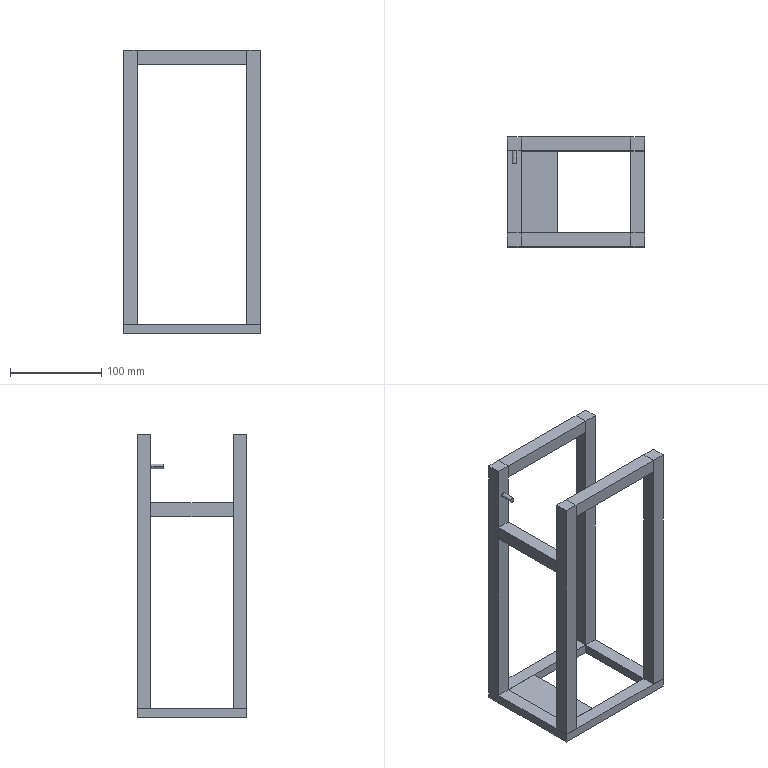Part | SolidWorks | features ICE 6, Extrusion 1 | 9 solids | 61 faces | box 150 x 120 x 310 mm | volume 427325 mm3 | plane 59 | cylinder 2 | commonest cylinder face diameters 5 x2
STEP:
#1=CARTESIAN_POINT('',(75.,-60.,0.));
#2=VERTEX_POINT('',#1);
#3=CARTESIAN_POINT('',(75.,60.,0.));
#4=VERTEX_POINT('',#3);
#5=CARTESIAN_POINT('',(75.,60.,0.));
#6=DIRECTION('',(0.,1.,0.));
#7=VECTOR('',#6,1000.);
#8=LINE('',#5,#7);
#9=EDGE_CURVE('',#2,#4,#8,.T.);
#10=ORIENTED_EDGE('',*,*,#9,.T.);
#11=CARTESIAN_POINT('',(75.,60.,10.));
#12=VERTEX_POINT('',#11);
#13=CARTESIAN_POINT('',(75.,60.,10.));
#14=DIRECTION('',(0.,0.,-1.));
#15=VECTOR('',#14,1000.);
#16=LINE('',#13,#15);
#17=EDGE_CURVE('',#12,#4,#16,.T.);
#18=ORIENTED_EDGE('',*,*,#17,.F.);
#19=CARTESIAN_POINT('',(75.,-60.,10.));
#20=VERTEX_POINT('',#19);
#21=CARTESIAN_POINT('',(75.,60.,10.));
#22=DIRECTION('',(0.,1.,0.));
#23=VECTOR('',#22,1000.);
#24=LINE('',#21,#23);
#25=EDGE_CURVE('',#20,#12,#24,.T.);
#26=ORIENTED_EDGE('',*,*,#25,.F.);
#27=CARTESIAN_POINT('',(75.,-60.,10.));
#28=DIRECTION('',(0.,0.,-1.));
#29=VECTOR('',#28,1000.);
#30=LINE('',#27,#29);
#31=EDGE_CURVE('',#20,#2,#30,.T.);
#32=ORIENTED_EDGE('',*,*,#31,.T.);
#33=EDGE_LOOP('',(#10,#18,#26,#32));
#34=FACE_OUTER_BOUND('',#33,.T.);
#35=CARTESIAN_POINT('',(75.,60.,10.));
#36=DIRECTION('',(-1.,0.,0.));
#37=DIRECTION('',(0.,-1.,0.));
#38=AXIS2_PLACEMENT_3D('',#35,#36,#37);
#39=PLANE('',#38);
#40=ADVANCED_FACE('',(#34),#39,.F.);
#41=CARTESIAN_POINT('',(-75.,60.,0.));
#42=VERTEX_POINT('',#41);
#43=CARTESIAN_POINT('',(-75.,60.,0.));
#44=DIRECTION('',(-1.,0.,0.));
#45=VECTOR('',#44,1000.);
#46=LINE('',#43,#45);
#47=EDGE_CURVE('',#4,#42,#46,.T.);
#48=ORIENTED_EDGE('',*,*,#47,.T.);
#49=CARTESIAN_POINT('',(-75.,60.,10.));
#50=VERTEX_POINT('',#49);
#51=CARTESIAN_POINT('',(-75.,60.,10.));
#52=DIRECTION('',(0.,0.,-1.));
#53=VECTOR('',#52,1000.);
#54=LINE('',#51,#53);
#55=EDGE_CURVE('',#50,#42,#54,.T.);
#56=ORIENTED_EDGE('',*,*,#55,.F.);
#57=CARTESIAN_POINT('',(-75.,60.,10.));
#58=DIRECTION('',(-1.,0.,0.));
#59=VECTOR('',#58,1000.);
#60=LINE('',#57,#59);
#61=EDGE_CURVE('',#12,#50,#60,.T.);
#62=ORIENTED_EDGE('',*,*,#61,.F.);
#63=ORIENTED_EDGE('',*,*,#17,.T.);
#64=EDGE_LOOP('',(#48,#56,#62,#63));
#65=FACE_OUTER_BOUND('',#64,.T.);
#66=CARTESIAN_POINT('',(-75.,60.,10.));
#67=DIRECTION('',(0.,-1.,0.));
#68=DIRECTION('',(0.,0.,-1.));
#69=AXIS2_PLACEMENT_3D('',#66,#67,#68);
#70=PLANE('',#69);
#71=ADVANCED_FACE('',(#65),#70,.F.);
#72=CARTESIAN_POINT('',(-75.,-60.,0.));
#73=VERTEX_POINT('',#72);
#74=CARTESIAN_POINT('',(-75.,60.,0.));
#75=DIRECTION('',(0.,-1.,0.));
#76=VECTOR('',#75,1000.);
#77=LINE('',#74,#76);
#78=EDGE_CURVE('',#42,#73,#77,.T.);
#79=ORIENTED_EDGE('',*,*,#78,.T.);
#80=CARTESIAN_POINT('',(-75.,-60.,10.));
#81=VERTEX_POINT('',#80);
#82=CARTESIAN_POINT('',(-75.,-60.,10.));
#83=DIRECTION('',(0.,0.,-1.));
#84=VECTOR('',#83,1000.);
#85=LINE('',#82,#84);
#86=EDGE_CURVE('',#81,#73,#85,.T.);
#87=ORIENTED_EDGE('',*,*,#86,.F.);
#88=CARTESIAN_POINT('',(-75.,60.,10.));
#89=DIRECTION('',(0.,-1.,0.));
#90=VECTOR('',#89,1000.);
#91=LINE('',#88,#90);
#92=EDGE_CURVE('',#50,#81,#91,.T.);
#93=ORIENTED_EDGE('',*,*,#92,.F.);
#94=ORIENTED_EDGE('',*,*,#55,.T.);
#95=EDGE_LOOP('',(#79,#87,#93,#94));
#96=FACE_OUTER_BOUND('',#95,.T.);
#97=CARTESIAN_POINT('',(-75.,60.,10.));
#98=DIRECTION('',(1.,0.,0.));
#99=DIRECTION('',(0.,1.,0.));
#100=AXIS2_PLACEMENT_3D('',#97,#98,#99);
#101=PLANE('',#100);
#102=ADVANCED_FACE('',(#96),#101,.F.);
#103=CARTESIAN_POINT('',(-75.,-60.,0.));
#104=DIRECTION('',(1.,0.,0.));
#105=VECTOR('',#104,1000.);
#106=LINE('',#103,#105);
#107=EDGE_CURVE('',#73,#2,#106,.T.);
#108=ORIENTED_EDGE('',*,*,#107,.T.);
#109=ORIENTED_EDGE('',*,*,#31,.F.);
#110=CARTESIAN_POINT('',(-75.,-60.,10.));
#111=DIRECTION('',(1.,0.,0.));
#112=VECTOR('',#111,1000.);
#113=LINE('',#110,#112);
#114=EDGE_CURVE('',#81,#20,#113,.T.);
#115=ORIENTED_EDGE('',*,*,#114,.F.);
#116=ORIENTED_EDGE('',*,*,#86,.T.);
#117=EDGE_LOOP('',(#108,#109,#115,#116));
#118=FACE_OUTER_BOUND('',#117,.T.);
#119=CARTESIAN_POINT('',(-75.,-60.,10.));
#120=DIRECTION('',(0.,1.,0.));
#121=DIRECTION('',(0.,0.,1.));
#122=AXIS2_PLACEMENT_3D('',#119,#120,#121);
#123=PLANE('',#122);
#124=ADVANCED_FACE('',(#118),#123,.F.);
#125=CARTESIAN_POINT('',(60.,-45.,10.));
#126=VERTEX_POINT('',#125);
#127=CARTESIAN_POINT('',(60.,45.,10.));
#128=VERTEX_POINT('',#127);
#129=CARTESIAN_POINT('',(60.,0.,10.));
#130=DIRECTION('',(0.,1.,0.));
#131=VECTOR('',#130,1000.);
#132=LINE('',#129,#131);
#133=EDGE_CURVE('',#126,#128,#132,.T.);
#134=ORIENTED_EDGE('',*,*,#133,.F.);
#135=CARTESIAN_POINT('',(-60.,-45.,10.));
#136=VERTEX_POINT('',#135);
#137=CARTESIAN_POINT('',(0.,-45.,10.));
#138=DIRECTION('',(1.,0.,0.));
#139=VECTOR('',#138,1000.);
#140=LINE('',#137,#139);
#141=EDGE_CURVE('',#136,#126,#140,.T.);
#142=ORIENTED_EDGE('',*,*,#141,.F.);
#143=CARTESIAN_POINT('',(-60.,45.,10.));
#144=VERTEX_POINT('',#143);
#145=CARTESIAN_POINT('',(-60.,0.,10.));
#146=DIRECTION('',(0.,-1.,0.));
#147=VECTOR('',#146,1000.);
#148=LINE('',#145,#147);
#149=EDGE_CURVE('',#144,#136,#148,.T.);
#150=ORIENTED_EDGE('',*,*,#149,.F.);
#151=CARTESIAN_POINT('',(0.,45.,10.));
#152=DIRECTION('',(-1.,0.,0.));
#153=VECTOR('',#152,1000.);
#154=LINE('',#151,#153);
#155=EDGE_CURVE('',#128,#144,#154,.T.);
#156=ORIENTED_EDGE('',*,*,#155,.F.);
#157=EDGE_LOOP('',(#134,#142,#150,#156));
#158=FACE_BOUND('',#157,.T.);
#159=ORIENTED_EDGE('',*,*,#25,.T.);
#160=ORIENTED_EDGE('',*,*,#61,.T.);
#161=ORIENTED_EDGE('',*,*,#92,.T.);
#162=ORIENTED_EDGE('',*,*,#114,.T.);
#163=EDGE_LOOP('',(#159,#160,#161,#162));
#164=FACE_OUTER_BOUND('',#163,.T.);
#165=CARTESIAN_POINT('',(0.,0.,10.));
#166=DIRECTION('',(0.,0.,1.));
#167=DIRECTION('',(1.,0.,0.));
#168=AXIS2_PLACEMENT_3D('',#165,#166,#167);
#169=PLANE('',#168);
#170=ADVANCED_FACE('',(#158,#164),#169,.T.);
#171=CARTESIAN_POINT('',(-60.,-45.,0.));
#172=VERTEX_POINT('',#171);
#173=CARTESIAN_POINT('',(60.,-45.,0.));
#174=VERTEX_POINT('',#173);
#175=CARTESIAN_POINT('',(-60.,-45.,0.));
#176=DIRECTION('',(1.,0.,0.));
#177=VECTOR('',#176,1000.);
#178=LINE('',#175,#177);
#179=EDGE_CURVE('',#172,#174,#178,.T.);
#180=ORIENTED_EDGE('',*,*,#179,.T.);
#181=CARTESIAN_POINT('',(60.,45.,0.));
#182=VERTEX_POINT('',#181);
#183=CARTESIAN_POINT('',(60.,45.,0.));
#184=DIRECTION('',(0.,1.,0.));
#185=VECTOR('',#184,1000.);
#186=LINE('',#183,#185);
#187=EDGE_CURVE('',#174,#182,#186,.T.);
#188=ORIENTED_EDGE('',*,*,#187,.T.);
#189=CARTESIAN_POINT('',(-60.,45.,0.));
#190=VERTEX_POINT('',#189);
#191=CARTESIAN_POINT('',(-60.,45.,0.));
#192=DIRECTION('',(-1.,0.,0.));
#193=VECTOR('',#192,1000.);
#194=LINE('',#191,#193);
#195=EDGE_CURVE('',#182,#190,#194,.T.);
#196=ORIENTED_EDGE('',*,*,#195,.T.);
#197=CARTESIAN_POINT('',(-60.,45.,0.));
#198=DIRECTION('',(0.,-1.,0.));
#199=VECTOR('',#198,1000.);
#200=LINE('',#197,#199);
#201=EDGE_CURVE('',#190,#172,#200,.T.);
#202=ORIENTED_EDGE('',*,*,#201,.T.);
#203=EDGE_LOOP('',(#180,#188,#196,#202));
#204=FACE_BOUND('',#203,.T.);
#205=ORIENTED_EDGE('',*,*,#9,.F.);
#206=ORIENTED_EDGE('',*,*,#107,.F.);
#207=ORIENTED_EDGE('',*,*,#78,.F.);
#208=ORIENTED_EDGE('',*,*,#47,.F.);
#209=EDGE_LOOP('',(#205,#206,#207,#208));
#210=FACE_OUTER_BOUND('',#209,.T.);
#211=CARTESIAN_POINT('',(0.,0.,0.));
#212=DIRECTION('',(0.,0.,1.));
#213=DIRECTION('',(1.,0.,0.));
#214=AXIS2_PLACEMENT_3D('',#211,#212,#213);
#215=PLANE('',#214);
#216=ADVANCED_FACE('',(#204,#210),#215,.F.);
#217=ORIENTED_EDGE('',*,*,#133,.T.);
#218=CARTESIAN_POINT('',(60.,45.,0.));
#219=DIRECTION('',(0.,0.,1.));
#220=VECTOR('',#219,1000.);
#221=LINE('',#218,#220);
#222=EDGE_CURVE('',#182,#128,#221,.T.);
#223=ORIENTED_EDGE('',*,*,#222,.F.);
#224=ORIENTED_EDGE('',*,*,#187,.F.);
#225=CARTESIAN_POINT('',(60.,-45.,0.));
#226=DIRECTION('',(0.,0.,1.));
#227=VECTOR('',#226,1000.);
#228=LINE('',#225,#227);
#229=EDGE_CURVE('',#174,#126,#228,.T.);
#230=ORIENTED_EDGE('',*,*,#229,.T.);
#231=EDGE_LOOP('',(#217,#223,#224,#230));
#232=FACE_OUTER_BOUND('',#231,.T.);
#233=CARTESIAN_POINT('',(60.,45.,0.));
#234=DIRECTION('',(1.,0.,0.));
#235=DIRECTION('',(0.,0.,-1.));
#236=AXIS2_PLACEMENT_3D('',#233,#234,#235);
#237=PLANE('',#236);
#238=ADVANCED_FACE('',(#232),#237,.F.);
#239=ORIENTED_EDGE('',*,*,#141,.T.);
#240=ORIENTED_EDGE('',*,*,#229,.F.);
#241=ORIENTED_EDGE('',*,*,#179,.F.);
#242=CARTESIAN_POINT('',(-60.,-45.,0.));
#243=DIRECTION('',(0.,0.,1.));
#244=VECTOR('',#243,1000.);
#245=LINE('',#242,#244);
#246=EDGE_CURVE('',#172,#136,#245,.T.);
#247=ORIENTED_EDGE('',*,*,#246,.T.);
#248=EDGE_LOOP('',(#239,#240,#241,#247));
#249=FACE_OUTER_BOUND('',#248,.T.);
#250=CARTESIAN_POINT('',(-60.,-45.,0.));
#251=DIRECTION('',(0.,-1.,0.));
#252=DIRECTION('',(0.,0.,-1.));
#253=AXIS2_PLACEMENT_3D('',#250,#251,#252);
#254=PLANE('',#253);
#255=ADVANCED_FACE('',(#249),#254,.F.);
#256=ORIENTED_EDGE('',*,*,#149,.T.);
#257=ORIENTED_EDGE('',*,*,#246,.F.);
#258=ORIENTED_EDGE('',*,*,#201,.F.);
#259=CARTESIAN_POINT('',(-60.,45.,0.));
#260=DIRECTION('',(0.,0.,1.));
#261=VECTOR('',#260,1000.);
#262=LINE('',#259,#261);
#263=EDGE_CURVE('',#190,#144,#262,.T.);
#264=ORIENTED_EDGE('',*,*,#263,.T.);
#265=EDGE_LOOP('',(#256,#257,#258,#264));
#266=FACE_OUTER_BOUND('',#265,.T.);
#267=CARTESIAN_POINT('',(-60.,45.,0.));
#268=DIRECTION('',(-1.,0.,0.));
#269=DIRECTION('',(0.,0.,1.));
#270=AXIS2_PLACEMENT_3D('',#267,#268,#269);
#271=PLANE('',#270);
#272=ADVANCED_FACE('',(#266),#271,.F.);
#273=ORIENTED_EDGE('',*,*,#155,.T.);
#274=ORIENTED_EDGE('',*,*,#263,.F.);
#275=ORIENTED_EDGE('',*,*,#195,.F.);
#276=ORIENTED_EDGE('',*,*,#222,.T.);
#277=EDGE_LOOP('',(#273,#274,#275,#276));
#278=FACE_OUTER_BOUND('',#277,.T.);
#279=CARTESIAN_POINT('',(-60.,45.,0.));
#280=DIRECTION('',(0.,1.,0.));
#281=DIRECTION('',(0.,0.,1.));
#282=AXIS2_PLACEMENT_3D('',#279,#280,#281);
#283=PLANE('',#282);
#284=ADVANCED_FACE('',(#278),#283,.F.);
#285=CLOSED_SHELL('',(#40,#71,#102,#124,#170,#216,#238,#255,#272,#284));
#286=MANIFOLD_SOLID_BREP('',#285);
#287=CARTESIAN_POINT('',(-75.,-45.,10.));
#288=VERTEX_POINT('',#287);
#289=CARTESIAN_POINT('',(-75.,-60.,10.));
#290=VERTEX_POINT('',#289);
#291=CARTESIAN_POINT('',(-75.,-60.,10.));
#292=DIRECTION('',(0.,-1.,0.));
#293=VECTOR('',#292,1000.);
#294=LINE('',#291,#293);
#295=EDGE_CURVE('',#288,#290,#294,.T.);
#296=ORIENTED_EDGE('',*,*,#295,.T.);
#297=CARTESIAN_POINT('',(-75.,-60.,310.));
#298=VERTEX_POINT('',#297);
#299=CARTESIAN_POINT('',(-75.,-60.,310.));
#300=DIRECTION('',(0.,0.,-1.));
#301=VECTOR('',#300,1000.);
#302=LINE('',#299,#301);
#303=EDGE_CURVE('',#298,#290,#302,.T.);
#304=ORIENTED_EDGE('',*,*,#303,.F.);
#305=CARTESIAN_POINT('',(-75.,-45.,310.));
#306=VERTEX_POINT('',#305);
#307=CARTESIAN_POINT('',(-75.,-60.,310.));
#308=DIRECTION('',(0.,-1.,0.));
#309=VECTOR('',#308,1000.);
#310=LINE('',#307,#309);
#311=EDGE_CURVE('',#306,#298,#310,.T.);
#312=ORIENTED_EDGE('',*,*,#311,.F.);
#313=CARTESIAN_POINT('',(-75.,-45.,310.));
#314=DIRECTION('',(0.,0.,-1.));
#315=VECTOR('',#314,1000.);
#316=LINE('',#313,#315);
#317=EDGE_CURVE('',#306,#288,#316,.T.);
#318=ORIENTED_EDGE('',*,*,#317,.T.);
#319=EDGE_LOOP('',(#296,#304,#312,#318));
#320=FACE_OUTER_BOUND('',#319,.T.);
#321=CARTESIAN_POINT('',(-75.,-60.,310.));
#322=DIRECTION('',(1.,0.,0.));
#323=DIRECTION('',(0.,0.,-1.));
#324=AXIS2_PLACEMENT_3D('',#321,#322,#323);
#325=PLANE('',#324);
#326=ADVANCED_FACE('',(#320),#325,.F.);
#327=CARTESIAN_POINT('',(-60.,-60.,10.));
#328=VERTEX_POINT('',#327);
#329=CARTESIAN_POINT('',(-75.,-60.,10.));
#330=DIRECTION('',(1.,0.,0.));
#331=VECTOR('',#330,1000.);
#332=LINE('',#329,#331);
#333=EDGE_CURVE('',#290,#328,#332,.T.);
#334=ORIENTED_EDGE('',*,*,#333,.T.);
#335=CARTESIAN_POINT('',(-60.,-60.,310.));
#336=VERTEX_POINT('',#335);
#337=CARTESIAN_POINT('',(-60.,-60.,310.));
#338=DIRECTION('',(0.,0.,-1.));
#339=VECTOR('',#338,1000.);
#340=LINE('',#337,#339);
#341=EDGE_CURVE('',#336,#328,#340,.T.);
#342=ORIENTED_EDGE('',*,*,#341,.F.);
#343=CARTESIAN_POINT('',(-75.,-60.,310.));
#344=DIRECTION('',(1.,0.,0.));
#345=VECTOR('',#344,1000.);
#346=LINE('',#343,#345);
#347=EDGE_CURVE('',#298,#336,#346,.T.);
#348=ORIENTED_EDGE('',*,*,#347,.F.);
#349=ORIENTED_EDGE('',*,*,#303,.T.);
#350=EDGE_LOOP('',(#334,#342,#348,#349));
#351=FACE_OUTER_BOUND('',#350,.T.);
#352=CARTESIAN_POINT('',(-75.,-60.,310.));
#353=DIRECTION('',(0.,1.,0.));
#354=DIRECTION('',(0.,0.,1.));
#355=AXIS2_PLACEMENT_3D('',#352,#353,#354);
#356=PLANE('',#355);
#357=ADVANCED_FACE('',(#351),#356,.F.);
#358=CARTESIAN_POINT('',(-60.,-45.,10.));
#359=VERTEX_POINT('',#358);
#360=CARTESIAN_POINT('',(-60.,-60.,10.));
#361=DIRECTION('',(0.,1.,0.));
#362=VECTOR('',#361,1000.);
#363=LINE('',#360,#362);
#364=EDGE_CURVE('',#328,#359,#363,.T.);
#365=ORIENTED_EDGE('',*,*,#364,.T.);
#366=CARTESIAN_POINT('',(-60.,-45.,310.));
#367=VERTEX_POINT('',#366);
#368=CARTESIAN_POINT('',(-60.,-45.,310.));
#369=DIRECTION('',(0.,0.,-1.));
#370=VECTOR('',#369,1000.);
#371=LINE('',#368,#370);
#372=EDGE_CURVE('',#367,#359,#371,.T.);
#373=ORIENTED_EDGE('',*,*,#372,.F.);
#374=CARTESIAN_POINT('',(-60.,-60.,310.));
#375=DIRECTION('',(0.,1.,0.));
#376=VECTOR('',#375,1000.);
#377=LINE('',#374,#376);
#378=EDGE_CURVE('',#336,#367,#377,.T.);
#379=ORIENTED_EDGE('',*,*,#378,.F.);
#380=ORIENTED_EDGE('',*,*,#341,.T.);
#381=EDGE_LOOP('',(#365,#373,#379,#380));
#382=FACE_OUTER_BOUND('',#381,.T.);
#383=CARTESIAN_POINT('',(-60.,-60.,310.));
#384=DIRECTION('',(-1.,0.,0.));
#385=DIRECTION('',(0.,0.,1.));
#386=AXIS2_PLACEMENT_3D('',#383,#384,#385);
#387=PLANE('',#386);
#388=ADVANCED_FACE('',(#382),#387,.F.);
#389=CARTESIAN_POINT('',(-75.,-45.,10.));
#390=DIRECTION('',(-1.,0.,0.));
#391=VECTOR('',#390,1000.);
#392=LINE('',#389,#391);
#393=EDGE_CURVE('',#359,#288,#392,.T.);
#394=ORIENTED_EDGE('',*,*,#393,.T.);
#395=ORIENTED_EDGE('',*,*,#317,.F.);
#396=CARTESIAN_POINT('',(-75.,-45.,310.));
#397=DIRECTION('',(-1.,0.,0.));
#398=VECTOR('',#397,1000.);
#399=LINE('',#396,#398);
#400=EDGE_CURVE('',#367,#306,#399,.T.);
#401=ORIENTED_EDGE('',*,*,#400,.F.);
#402=ORIENTED_EDGE('',*,*,#372,.T.);
#403=EDGE_LOOP('',(#394,#395,#401,#402));
#404=FACE_OUTER_BOUND('',#403,.T.);
#405=CARTESIAN_POINT('',(-75.,-45.,310.));
#406=DIRECTION('',(0.,-1.,0.));
#407=DIRECTION('',(1.,0.,0.));
#408=AXIS2_PLACEMENT_3D('',#405,#406,#407);
#409=PLANE('',#408);
#410=ADVANCED_FACE('',(#404),#409,.F.);
#411=ORIENTED_EDGE('',*,*,#311,.T.);
#412=ORIENTED_EDGE('',*,*,#347,.T.);
#413=ORIENTED_EDGE('',*,*,#378,.T.);
#414=ORIENTED_EDGE('',*,*,#400,.T.);
#415=EDGE_LOOP('',(#411,#412,#413,#414));
#416=FACE_OUTER_BOUND('',#415,.T.);
#417=CARTESIAN_POINT('',(0.,0.,310.));
#418=DIRECTION('',(0.,0.,-1.));
#419=DIRECTION('',(-1.,0.,0.));
#420=AXIS2_PLACEMENT_3D('',#417,#418,#419);
#421=PLANE('',#420);
#422=ADVANCED_FACE('',(#416),#421,.F.);
#423=ORIENTED_EDGE('',*,*,#295,.F.);
#424=ORIENTED_EDGE('',*,*,#393,.F.);
#425=ORIENTED_EDGE('',*,*,#364,.F.);
#426=ORIENTED_EDGE('',*,*,#333,.F.);
#427=EDGE_LOOP('',(#423,#424,#425,#426));
#428=FACE_OUTER_BOUND('',#427,.T.);
#429=CARTESIAN_POINT('',(0.,0.,10.));
#430=DIRECTION('',(0.,0.,-1.));
#431=DIRECTION('',(-1.,0.,0.));
#432=AXIS2_PLACEMENT_3D('',#429,#430,#431);
#433=PLANE('',#432);
#434=ADVANCED_FACE('',(#428),#433,.T.);
#435=CLOSED_SHELL('',(#326,#357,#388,#410,#422,#434));
#436=MANIFOLD_SOLID_BREP('',#435);
#437=CARTESIAN_POINT('',(75.,45.,10.));
#438=VERTEX_POINT('',#437);
#439=CARTESIAN_POINT('',(75.,60.,10.));
#440=VERTEX_POINT('',#439);
#441=CARTESIAN_POINT('',(75.,60.,10.));
#442=DIRECTION('',(0.,1.,0.));
#443=VECTOR('',#442,1000.);
#444=LINE('',#441,#443);
#445=EDGE_CURVE('',#438,#440,#444,.T.);
#446=ORIENTED_EDGE('',*,*,#445,.T.);
#447=CARTESIAN_POINT('',(75.,60.,310.));
#448=VERTEX_POINT('',#447);
#449=CARTESIAN_POINT('',(75.,60.,310.));
#450=DIRECTION('',(0.,0.,-1.));
#451=VECTOR('',#450,1000.);
#452=LINE('',#449,#451);
#453=EDGE_CURVE('',#448,#440,#452,.T.);
#454=ORIENTED_EDGE('',*,*,#453,.F.);
#455=CARTESIAN_POINT('',(75.,45.,310.));
#456=VERTEX_POINT('',#455);
#457=CARTESIAN_POINT('',(75.,60.,310.));
#458=DIRECTION('',(0.,1.,0.));
#459=VECTOR('',#458,1000.);
#460=LINE('',#457,#459);
#461=EDGE_CURVE('',#456,#448,#460,.T.);
#462=ORIENTED_EDGE('',*,*,#461,.F.);
#463=CARTESIAN_POINT('',(75.,45.,310.));
#464=DIRECTION('',(0.,0.,-1.));
#465=VECTOR('',#464,1000.);
#466=LINE('',#463,#465);
#467=EDGE_CURVE('',#456,#438,#466,.T.);
#468=ORIENTED_EDGE('',*,*,#467,.T.);
#469=EDGE_LOOP('',(#446,#454,#462,#468));
#470=FACE_OUTER_BOUND('',#469,.T.);
#471=CARTESIAN_POINT('',(75.,60.,310.));
#472=DIRECTION('',(-1.,0.,0.));
#473=DIRECTION('',(0.,-1.,0.));
#474=AXIS2_PLACEMENT_3D('',#471,#472,#473);
#475=PLANE('',#474);
#476=ADVANCED_FACE('',(#470),#475,.F.);
#477=CARTESIAN_POINT('',(60.,60.,10.));
#478=VERTEX_POINT('',#477);
#479=CARTESIAN_POINT('',(75.,60.,10.));
#480=DIRECTION('',(-1.,0.,0.));
#481=VECTOR('',#480,1000.);
#482=LINE('',#479,#481);
#483=EDGE_CURVE('',#440,#478,#482,.T.);
#484=ORIENTED_EDGE('',*,*,#483,.T.);
#485=CARTESIAN_POINT('',(60.,60.,310.));
#486=VERTEX_POINT('',#485);
#487=CARTESIAN_POINT('',(60.,60.,310.));
#488=DIRECTION('',(0.,0.,-1.));
#489=VECTOR('',#488,1000.);
#490=LINE('',#487,#489);
#491=EDGE_CURVE('',#486,#478,#490,.T.);
#492=ORIENTED_EDGE('',*,*,#491,.F.);
#493=CARTESIAN_POINT('',(75.,60.,310.));
#494=DIRECTION('',(-1.,0.,0.));
#495=VECTOR('',#494,1000.);
#496=LINE('',#493,#495);
#497=EDGE_CURVE('',#448,#486,#496,.T.);
#498=ORIENTED_EDGE('',*,*,#497,.F.);
#499=ORIENTED_EDGE('',*,*,#453,.T.);
#500=EDGE_LOOP('',(#484,#492,#498,#499));
#501=FACE_OUTER_BOUND('',#500,.T.);
#502=CARTESIAN_POINT('',(75.,60.,310.));
#503=DIRECTION('',(0.,-1.,0.));
#504=DIRECTION('',(0.,0.,-1.));
#505=AXIS2_PLACEMENT_3D('',#502,#503,#504);
#506=PLANE('',#505);
#507=ADVANCED_FACE('',(#501),#506,.F.);
#508=CARTESIAN_POINT('',(60.,45.,10.));
#509=VERTEX_POINT('',#508);
#510=CARTESIAN_POINT('',(60.,60.,10.));
#511=DIRECTION('',(0.,-1.,0.));
#512=VECTOR('',#511,1000.);
#513=LINE('',#510,#512);
#514=EDGE_CURVE('',#478,#509,#513,.T.);
#515=ORIENTED_EDGE('',*,*,#514,.T.);
#516=CARTESIAN_POINT('',(60.,45.,310.));
#517=VERTEX_POINT('',#516);
#518=CARTESIAN_POINT('',(60.,45.,310.));
#519=DIRECTION('',(0.,0.,-1.));
#520=VECTOR('',#519,1000.);
#521=LINE('',#518,#520);
#522=EDGE_CURVE('',#517,#509,#521,.T.);
#523=ORIENTED_EDGE('',*,*,#522,.F.);
#524=CARTESIAN_POINT('',(60.,60.,310.));
#525=DIRECTION('',(0.,-1.,0.));
#526=VECTOR('',#525,1000.);
#527=LINE('',#524,#526);
#528=EDGE_CURVE('',#486,#517,#527,.T.);
#529=ORIENTED_EDGE('',*,*,#528,.F.);
#530=ORIENTED_EDGE('',*,*,#491,.T.);
#531=EDGE_LOOP('',(#515,#523,#529,#530));
#532=FACE_OUTER_BOUND('',#531,.T.);
#533=CARTESIAN_POINT('',(60.,60.,310.));
#534=DIRECTION('',(1.,0.,0.));
#535=DIRECTION('',(0.,1.,0.));
#536=AXIS2_PLACEMENT_3D('',#533,#534,#535);
#537=PLANE('',#536);
#538=ADVANCED_FACE('',(#532),#537,.F.);
#539=CARTESIAN_POINT('',(75.,45.,10.));
#540=DIRECTION('',(1.,0.,0.));
#541=VECTOR('',#540,1000.);
#542=LINE('',#539,#541);
#543=EDGE_CURVE('',#509,#438,#542,.T.);
#544=ORIENTED_EDGE('',*,*,#543,.T.);
#545=ORIENTED_EDGE('',*,*,#467,.F.);
#546=CARTESIAN_POINT('',(75.,45.,310.));
#547=DIRECTION('',(1.,0.,0.));
#548=VECTOR('',#547,1000.);
#549=LINE('',#546,#548);
#550=EDGE_CURVE('',#517,#456,#549,.T.);
#551=ORIENTED_EDGE('',*,*,#550,.F.);
#552=ORIENTED_EDGE('',*,*,#522,.T.);
#553=EDGE_LOOP('',(#544,#545,#551,#552));
#554=FACE_OUTER_BOUND('',#553,.T.);
#555=CARTESIAN_POINT('',(75.,45.,310.));
#556=DIRECTION('',(0.,1.,0.));
#557=DIRECTION('',(0.,0.,1.));
#558=AXIS2_PLACEMENT_3D('',#555,#556,#557);
#559=PLANE('',#558);
#560=ADVANCED_FACE('',(#554),#559,.F.);
#561=ORIENTED_EDGE('',*,*,#461,.T.);
#562=ORIENTED_EDGE('',*,*,#497,.T.);
#563=ORIENTED_EDGE('',*,*,#528,.T.);
#564=ORIENTED_EDGE('',*,*,#550,.T.);
#565=EDGE_LOOP('',(#561,#562,#563,#564));
#566=FACE_OUTER_BOUND('',#565,.T.);
#567=CARTESIAN_POINT('',(0.,0.,310.));
#568=DIRECTION('',(0.,0.,-1.));
#569=DIRECTION('',(-1.,0.,0.));
#570=AXIS2_PLACEMENT_3D('',#567,#568,#569);
#571=PLANE('',#570);
#572=ADVANCED_FACE('',(#566),#571,.F.);
#573=ORIENTED_EDGE('',*,*,#445,.F.);
#574=ORIENTED_EDGE('',*,*,#543,.F.);
#575=ORIENTED_EDGE('',*,*,#514,.F.);
#576=ORIENTED_EDGE('',*,*,#483,.F.);
#577=EDGE_LOOP('',(#573,#574,#575,#576));
#578=FACE_OUTER_BOUND('',#577,.T.);
#579=CARTESIAN_POINT('',(0.,0.,10.));
#580=DIRECTION('',(0.,0.,-1.));
#581=DIRECTION('',(-1.,0.,0.));
#582=AXIS2_PLACEMENT_3D('',#579,#580,#581);
#583=PLANE('',#582);
#584=ADVANCED_FACE('',(#578),#583,.T.);
#585=CLOSED_SHELL('',(#476,#507,#538,#560,#572,#584));
#586=MANIFOLD_SOLID_BREP('',#585);
#587=CARTESIAN_POINT('',(75.,-60.,10.));
#588=VERTEX_POINT('',#587);
#589=CARTESIAN_POINT('',(75.,-45.,10.));
#590=VERTEX_POINT('',#589);
#591=CARTESIAN_POINT('',(75.,-60.,10.));
#592=DIRECTION('',(0.,1.,0.));
#593=VECTOR('',#592,1000.);
#594=LINE('',#591,#593);
#595=EDGE_CURVE('',#588,#590,#594,.T.);
#596=ORIENTED_EDGE('',*,*,#595,.T.);
#597=CARTESIAN_POINT('',(75.,-45.,310.));
#598=VERTEX_POINT('',#597);
#599=CARTESIAN_POINT('',(75.,-45.,310.));
#600=DIRECTION('',(0.,0.,-1.));
#601=VECTOR('',#600,1000.);
#602=LINE('',#599,#601);
#603=EDGE_CURVE('',#598,#590,#602,.T.);
#604=ORIENTED_EDGE('',*,*,#603,.F.);
#605=CARTESIAN_POINT('',(75.,-60.,310.));
#606=VERTEX_POINT('',#605);
#607=CARTESIAN_POINT('',(75.,-60.,310.));
#608=DIRECTION('',(0.,1.,0.));
#609=VECTOR('',#608,1000.);
#610=LINE('',#607,#609);
#611=EDGE_CURVE('',#606,#598,#610,.T.);
#612=ORIENTED_EDGE('',*,*,#611,.F.);
#613=CARTESIAN_POINT('',(75.,-60.,310.));
#614=DIRECTION('',(0.,0.,-1.));
#615=VECTOR('',#614,1000.);
#616=LINE('',#613,#615);
#617=EDGE_CURVE('',#606,#588,#616,.T.);
#618=ORIENTED_EDGE('',*,*,#617,.T.);
#619=EDGE_LOOP('',(#596,#604,#612,#618));
#620=FACE_OUTER_BOUND('',#619,.T.);
#621=CARTESIAN_POINT('',(75.,-60.,310.));
#622=DIRECTION('',(-1.,0.,0.));
#623=DIRECTION('',(0.,0.,1.));
#624=AXIS2_PLACEMENT_3D('',#621,#622,#623);
#625=PLANE('',#624);
#626=ADVANCED_FACE('',(#620),#625,.F.);
#627=CARTESIAN_POINT('',(60.,-45.,10.));
#628=VERTEX_POINT('',#627);
#629=CARTESIAN_POINT('',(75.,-45.,10.));
#630=DIRECTION('',(-1.,0.,0.));
#631=VECTOR('',#630,1000.);
#632=LINE('',#629,#631);
#633=EDGE_CURVE('',#590,#628,#632,.T.);
#634=ORIENTED_EDGE('',*,*,#633,.T.);
#635=CARTESIAN_POINT('',(60.,-45.,310.));
#636=VERTEX_POINT('',#635);
#637=CARTESIAN_POINT('',(60.,-45.,310.));
#638=DIRECTION('',(0.,0.,-1.));
#639=VECTOR('',#638,1000.);
#640=LINE('',#637,#639);
#641=EDGE_CURVE('',#636,#628,#640,.T.);
#642=ORIENTED_EDGE('',*,*,#641,.F.);
#643=CARTESIAN_POINT('',(75.,-45.,310.));
#644=DIRECTION('',(-1.,0.,0.));
#645=VECTOR('',#644,1000.);
#646=LINE('',#643,#645);
#647=EDGE_CURVE('',#598,#636,#646,.T.);
#648=ORIENTED_EDGE('',*,*,#647,.F.);
#649=ORIENTED_EDGE('',*,*,#603,.T.);
#650=EDGE_LOOP('',(#634,#642,#648,#649));
#651=FACE_OUTER_BOUND('',#650,.T.);
#652=CARTESIAN_POINT('',(75.,-45.,310.));
#653=DIRECTION('',(0.,-1.,0.));
#654=DIRECTION('',(0.,0.,-1.));
#655=AXIS2_PLACEMENT_3D('',#652,#653,#654);
#656=PLANE('',#655);
#657=ADVANCED_FACE('',(#651),#656,.F.);
#658=CARTESIAN_POINT('',(60.,-60.,10.));
#659=VERTEX_POINT('',#658);
#660=CARTESIAN_POINT('',(60.,-60.,10.));
#661=DIRECTION('',(0.,-1.,0.));
#662=VECTOR('',#661,1000.);
#663=LINE('',#660,#662);
#664=EDGE_CURVE('',#628,#659,#663,.T.);
#665=ORIENTED_EDGE('',*,*,#664,.T.);
#666=CARTESIAN_POINT('',(60.,-60.,310.));
#667=VERTEX_POINT('',#666);
#668=CARTESIAN_POINT('',(60.,-60.,310.));
#669=DIRECTION('',(0.,0.,-1.));
#670=VECTOR('',#669,1000.);
#671=LINE('',#668,#670);
#672=EDGE_CURVE('',#667,#659,#671,.T.);
#673=ORIENTED_EDGE('',*,*,#672,.F.);
#674=CARTESIAN_POINT('',(60.,-60.,310.));
#675=DIRECTION('',(0.,-1.,0.));
#676=VECTOR('',#675,1000.);
#677=LINE('',#674,#676);
#678=EDGE_CURVE('',#636,#667,#677,.T.);
#679=ORIENTED_EDGE('',*,*,#678,.F.);
#680=ORIENTED_EDGE('',*,*,#641,.T.);
#681=EDGE_LOOP('',(#665,#673,#679,#680));
#682=FACE_OUTER_BOUND('',#681,.T.);
#683=CARTESIAN_POINT('',(60.,-60.,310.));
#684=DIRECTION('',(1.,0.,0.));
#685=DIRECTION('',(0.,0.,-1.));
#686=AXIS2_PLACEMENT_3D('',#683,#684,#685);
#687=PLANE('',#686);
#688=ADVANCED_FACE('',(#682),#687,.F.);
#689=CARTESIAN_POINT('',(75.,-60.,10.));
#690=DIRECTION('',(1.,0.,0.));
#691=VECTOR('',#690,1000.);
#692=LINE('',#689,#691);
#693=EDGE_CURVE('',#659,#588,#692,.T.);
#694=ORIENTED_EDGE('',*,*,#693,.T.);
#695=ORIENTED_EDGE('',*,*,#617,.F.);
#696=CARTESIAN_POINT('',(75.,-60.,310.));
#697=DIRECTION('',(1.,0.,0.));
#698=VECTOR('',#697,1000.);
#699=LINE('',#696,#698);
#700=EDGE_CURVE('',#667,#606,#699,.T.);
#701=ORIENTED_EDGE('',*,*,#700,.F.);
#702=ORIENTED_EDGE('',*,*,#672,.T.);
#703=EDGE_LOOP('',(#694,#695,#701,#702));
#704=FACE_OUTER_BOUND('',#703,.T.);
#705=CARTESIAN_POINT('',(75.,-60.,310.));
#706=DIRECTION('',(0.,1.,0.));
#707=DIRECTION('',(0.,0.,1.));
#708=AXIS2_PLACEMENT_3D('',#705,#706,#707);
#709=PLANE('',#708);
#710=ADVANCED_FACE('',(#704),#709,.F.);
#711=ORIENTED_EDGE('',*,*,#611,.T.);
#712=ORIENTED_EDGE('',*,*,#647,.T.);
#713=ORIENTED_EDGE('',*,*,#678,.T.);
#714=ORIENTED_EDGE('',*,*,#700,.T.);
#715=EDGE_LOOP('',(#711,#712,#713,#714));
#716=FACE_OUTER_BOUND('',#715,.T.);
#717=CARTESIAN_POINT('',(0.,0.,310.));
#718=DIRECTION('',(0.,0.,1.));
#719=DIRECTION('',(1.,0.,0.));
#720=AXIS2_PLACEMENT_3D('',#717,#718,#719);
#721=PLANE('',#720);
#722=ADVANCED_FACE('',(#716),#721,.T.);
#723=ORIENTED_EDGE('',*,*,#595,.F.);
#724=ORIENTED_EDGE('',*,*,#693,.F.);
#725=ORIENTED_EDGE('',*,*,#664,.F.);
#726=ORIENTED_EDGE('',*,*,#633,.F.);
#727=EDGE_LOOP('',(#723,#724,#725,#726));
#728=FACE_OUTER_BOUND('',#727,.T.);
#729=CARTESIAN_POINT('',(0.,0.,10.));
#730=DIRECTION('',(0.,0.,1.));
#731=DIRECTION('',(1.,0.,0.));
#732=AXIS2_PLACEMENT_3D('',#729,#730,#731);
#733=PLANE('',#732);
#734=ADVANCED_FACE('',(#728),#733,.F.);
#735=CLOSED_SHELL('',(#626,#657,#688,#710,#722,#734));
#736=MANIFOLD_SOLID_BREP('',#735);
#737=CARTESIAN_POINT('',(60.,60.,310.));
#738=VERTEX_POINT('',#737);
#739=CARTESIAN_POINT('',(60.,45.,310.));
#740=VERTEX_POINT('',#739);
#741=CARTESIAN_POINT('',(60.,60.,310.));
#742=DIRECTION('',(0.,-1.,0.));
#743=VECTOR('',#742,1000.);
#744=LINE('',#741,#743);
#745=EDGE_CURVE('',#738,#740,#744,.T.);
#746=ORIENTED_EDGE('',*,*,#745,.F.);
#747=CARTESIAN_POINT('',(-60.,60.,310.));
#748=VERTEX_POINT('',#747);
#749=CARTESIAN_POINT('',(81.213,60.,310.));
#750=DIRECTION('',(-1.,0.,0.));
#751=VECTOR('',#750,1000.);
#752=LINE('',#749,#751);
#753=EDGE_CURVE('',#738,#748,#752,.T.);
#754=ORIENTED_EDGE('',*,*,#753,.T.);
#755=CARTESIAN_POINT('',(-60.,45.,310.));
#756=VERTEX_POINT('',#755);
#757=CARTESIAN_POINT('',(-60.,60.,310.));
#758=DIRECTION('',(0.,-1.,0.));
#759=VECTOR('',#758,1000.);
#760=LINE('',#757,#759);
#761=EDGE_CURVE('',#748,#756,#760,.T.);
#762=ORIENTED_EDGE('',*,*,#761,.T.);
#763=CARTESIAN_POINT('',(81.213,45.,310.));
#764=DIRECTION('',(-1.,0.,0.));
#765=VECTOR('',#764,1000.);
#766=LINE('',#763,#765);
#767=EDGE_CURVE('',#740,#756,#766,.T.);
#768=ORIENTED_EDGE('',*,*,#767,.F.);
#769=EDGE_LOOP('',(#746,#754,#762,#768));
#770=FACE_OUTER_BOUND('',#769,.T.);
#771=CARTESIAN_POINT('',(81.213,60.,310.));
#772=DIRECTION('',(0.,0.,-1.));
#773=DIRECTION('',(-1.,0.,0.));
#774=AXIS2_PLACEMENT_3D('',#771,#772,#773);
#775=PLANE('',#774);
#776=ADVANCED_FACE('',(#770),#775,.F.);
#777=CARTESIAN_POINT('',(60.,45.,295.));
#778=VERTEX_POINT('',#777);
#779=CARTESIAN_POINT('',(60.,45.,310.));
#780=DIRECTION('',(0.,0.,-1.));
#781=VECTOR('',#780,1000.);
#782=LINE('',#779,#781);
#783=EDGE_CURVE('',#740,#778,#782,.T.);
#784=ORIENTED_EDGE('',*,*,#783,.F.);
#785=ORIENTED_EDGE('',*,*,#767,.T.);
#786=CARTESIAN_POINT('',(-60.,45.,295.));
#787=VERTEX_POINT('',#786);
#788=CARTESIAN_POINT('',(-60.,45.,310.));
#789=DIRECTION('',(0.,0.,-1.));
#790=VECTOR('',#789,1000.);
#791=LINE('',#788,#790);
#792=EDGE_CURVE('',#756,#787,#791,.T.);
#793=ORIENTED_EDGE('',*,*,#792,.T.);
#794=CARTESIAN_POINT('',(81.213,45.,295.));
#795=DIRECTION('',(-1.,0.,0.));
#796=VECTOR('',#795,1000.);
#797=LINE('',#794,#796);
#798=EDGE_CURVE('',#778,#787,#797,.T.);
#799=ORIENTED_EDGE('',*,*,#798,.F.);
#800=EDGE_LOOP('',(#784,#785,#793,#799));
#801=FACE_OUTER_BOUND('',#800,.T.);
#802=CARTESIAN_POINT('',(81.213,45.,310.));
#803=DIRECTION('',(0.,1.,0.));
#804=DIRECTION('',(0.,0.,1.));
#805=AXIS2_PLACEMENT_3D('',#802,#803,#804);
#806=PLANE('',#805);
#807=ADVANCED_FACE('',(#801),#806,.F.);
#808=CARTESIAN_POINT('',(60.,60.,295.));
#809=VERTEX_POINT('',#808);
#810=CARTESIAN_POINT('',(60.,60.,295.));
#811=DIRECTION('',(0.,1.,0.));
#812=VECTOR('',#811,1000.);
#813=LINE('',#810,#812);
#814=EDGE_CURVE('',#778,#809,#813,.T.);
#815=ORIENTED_EDGE('',*,*,#814,.F.);
#816=ORIENTED_EDGE('',*,*,#798,.T.);
#817=CARTESIAN_POINT('',(-60.,60.,295.));
#818=VERTEX_POINT('',#817);
#819=CARTESIAN_POINT('',(-60.,60.,295.));
#820=DIRECTION('',(0.,1.,0.));
#821=VECTOR('',#820,1000.);
#822=LINE('',#819,#821);
#823=EDGE_CURVE('',#787,#818,#822,.T.);
#824=ORIENTED_EDGE('',*,*,#823,.T.);
#825=CARTESIAN_POINT('',(81.213,60.,295.));
#826=DIRECTION('',(-1.,0.,0.));
#827=VECTOR('',#826,1000.);
#828=LINE('',#825,#827);
#829=EDGE_CURVE('',#809,#818,#828,.T.);
#830=ORIENTED_EDGE('',*,*,#829,.F.);
#831=EDGE_LOOP('',(#815,#816,#824,#830));
#832=FACE_OUTER_BOUND('',#831,.T.);
#833=CARTESIAN_POINT('',(81.213,60.,295.));
#834=DIRECTION('',(0.,0.,1.));
#835=DIRECTION('',(1.,0.,0.));
#836=AXIS2_PLACEMENT_3D('',#833,#834,#835);
#837=PLANE('',#836);
#838=ADVANCED_FACE('',(#832),#837,.F.);
#839=CARTESIAN_POINT('',(60.,60.,310.));
#840=DIRECTION('',(0.,0.,1.));
#841=VECTOR('',#840,1000.);
#842=LINE('',#839,#841);
#843=EDGE_CURVE('',#809,#738,#842,.T.);
#844=ORIENTED_EDGE('',*,*,#843,.F.);
#845=ORIENTED_EDGE('',*,*,#829,.T.);
#846=CARTESIAN_POINT('',(-60.,60.,310.));
#847=DIRECTION('',(0.,0.,1.));
#848=VECTOR('',#847,1000.);
#849=LINE('',#846,#848);
#850=EDGE_CURVE('',#818,#748,#849,.T.);
#851=ORIENTED_EDGE('',*,*,#850,.T.);
#852=ORIENTED_EDGE('',*,*,#753,.F.);
#853=EDGE_LOOP('',(#844,#845,#851,#852));
#854=FACE_OUTER_BOUND('',#853,.T.);
#855=CARTESIAN_POINT('',(81.213,60.,310.));
#856=DIRECTION('',(0.,-1.,0.));
#857=DIRECTION('',(0.,0.,-1.));
#858=AXIS2_PLACEMENT_3D('',#855,#856,#857);
#859=PLANE('',#858);
#860=ADVANCED_FACE('',(#854),#859,.F.);
#861=ORIENTED_EDGE('',*,*,#761,.F.);
#862=ORIENTED_EDGE('',*,*,#850,.F.);
#863=ORIENTED_EDGE('',*,*,#823,.F.);
#864=ORIENTED_EDGE('',*,*,#792,.F.);
#865=EDGE_LOOP('',(#861,#862,#863,#864));
#866=FACE_OUTER_BOUND('',#865,.T.);
#867=CARTESIAN_POINT('',(-60.,0.,0.));
#868=DIRECTION('',(1.,0.,0.));
#869=DIRECTION('',(0.,0.,-1.));
#870=AXIS2_PLACEMENT_3D('',#867,#868,#869);
#871=PLANE('',#870);
#872=ADVANCED_FACE('',(#866),#871,.F.);
#873=ORIENTED_EDGE('',*,*,#843,.T.);
#874=ORIENTED_EDGE('',*,*,#745,.T.);
#875=ORIENTED_EDGE('',*,*,#783,.T.);
#876=ORIENTED_EDGE('',*,*,#814,.T.);
#877=EDGE_LOOP('',(#873,#874,#875,#876));
#878=FACE_OUTER_BOUND('',#877,.T.);
#879=CARTESIAN_POINT('',(60.,-60.,310.));
#880=DIRECTION('',(1.,0.,0.));
#881=DIRECTION('',(0.,0.,-1.));
#882=AXIS2_PLACEMENT_3D('',#879,#880,#881);
#883=PLANE('',#882);
#884=ADVANCED_FACE('',(#878),#883,.T.);
#885=CLOSED_SHELL('',(#776,#807,#838,#860,#872,#884));
#886=MANIFOLD_SOLID_BREP('',#885);
#887=CARTESIAN_POINT('',(60.,-45.,310.));
#888=VERTEX_POINT('',#887);
#889=CARTESIAN_POINT('',(60.,-60.,310.));
#890=VERTEX_POINT('',#889);
#891=CARTESIAN_POINT('',(60.,-45.,310.));
#892=DIRECTION('',(0.,-1.,0.));
#893=VECTOR('',#892,1000.);
#894=LINE('',#891,#893);
#895=EDGE_CURVE('',#888,#890,#894,.T.);
#896=ORIENTED_EDGE('',*,*,#895,.F.);
#897=CARTESIAN_POINT('',(-60.,-45.,310.));
#898=VERTEX_POINT('',#897);
#899=CARTESIAN_POINT('',(81.213,-45.,310.));
#900=DIRECTION('',(-1.,0.,0.));
#901=VECTOR('',#900,1000.);
#902=LINE('',#899,#901);
#903=EDGE_CURVE('',#888,#898,#902,.T.);
#904=ORIENTED_EDGE('',*,*,#903,.T.);
#905=CARTESIAN_POINT('',(-60.,-60.,310.));
#906=VERTEX_POINT('',#905);
#907=CARTESIAN_POINT('',(-60.,-45.,310.));
#908=DIRECTION('',(0.,-1.,0.));
#909=VECTOR('',#908,1000.);
#910=LINE('',#907,#909);
#911=EDGE_CURVE('',#898,#906,#910,.T.);
#912=ORIENTED_EDGE('',*,*,#911,.T.);
#913=CARTESIAN_POINT('',(81.213,-60.,310.));
#914=DIRECTION('',(-1.,0.,0.));
#915=VECTOR('',#914,1000.);
#916=LINE('',#913,#915);
#917=EDGE_CURVE('',#890,#906,#916,.T.);
#918=ORIENTED_EDGE('',*,*,#917,.F.);
#919=EDGE_LOOP('',(#896,#904,#912,#918));
#920=FACE_OUTER_BOUND('',#919,.T.);
#921=CARTESIAN_POINT('',(81.213,-45.,310.));
#922=DIRECTION('',(0.,0.,-1.));
#923=DIRECTION('',(-1.,0.,0.));
#924=AXIS2_PLACEMENT_3D('',#921,#922,#923);
#925=PLANE('',#924);
#926=ADVANCED_FACE('',(#920),#925,.F.);
#927=CARTESIAN_POINT('',(60.,-60.,295.));
#928=VERTEX_POINT('',#927);
#929=CARTESIAN_POINT('',(60.,-60.,310.));
#930=DIRECTION('',(0.,0.,-1.));
#931=VECTOR('',#930,1000.);
#932=LINE('',#929,#931);
#933=EDGE_CURVE('',#890,#928,#932,.T.);
#934=ORIENTED_EDGE('',*,*,#933,.F.);
#935=ORIENTED_EDGE('',*,*,#917,.T.);
#936=CARTESIAN_POINT('',(-60.,-60.,295.));
#937=VERTEX_POINT('',#936);
#938=CARTESIAN_POINT('',(-60.,-60.,310.));
#939=DIRECTION('',(0.,0.,-1.));
#940=VECTOR('',#939,1000.);
#941=LINE('',#938,#940);
#942=EDGE_CURVE('',#906,#937,#941,.T.);
#943=ORIENTED_EDGE('',*,*,#942,.T.);
#944=CARTESIAN_POINT('',(81.213,-60.,295.));
#945=DIRECTION('',(-1.,0.,0.));
#946=VECTOR('',#945,1000.);
#947=LINE('',#944,#946);
#948=EDGE_CURVE('',#928,#937,#947,.T.);
#949=ORIENTED_EDGE('',*,*,#948,.F.);
#950=EDGE_LOOP('',(#934,#935,#943,#949));
#951=FACE_OUTER_BOUND('',#950,.T.);
#952=CARTESIAN_POINT('',(81.213,-60.,310.));
#953=DIRECTION('',(0.,1.,0.));
#954=DIRECTION('',(0.,0.,1.));
#955=AXIS2_PLACEMENT_3D('',#952,#953,#954);
#956=PLANE('',#955);
#957=ADVANCED_FACE('',(#951),#956,.F.);
#958=CARTESIAN_POINT('',(60.,-45.,295.));
#959=VERTEX_POINT('',#958);
#960=CARTESIAN_POINT('',(60.,-45.,295.));
#961=DIRECTION('',(0.,1.,0.));
#962=VECTOR('',#961,1000.);
#963=LINE('',#960,#962);
#964=EDGE_CURVE('',#928,#959,#963,.T.);
#965=ORIENTED_EDGE('',*,*,#964,.F.);
#966=ORIENTED_EDGE('',*,*,#948,.T.);
#967=CARTESIAN_POINT('',(-60.,-45.,295.));
#968=VERTEX_POINT('',#967);
#969=CARTESIAN_POINT('',(-60.,-45.,295.));
#970=DIRECTION('',(0.,1.,0.));
#971=VECTOR('',#970,1000.);
#972=LINE('',#969,#971);
#973=EDGE_CURVE('',#937,#968,#972,.T.);
#974=ORIENTED_EDGE('',*,*,#973,.T.);
#975=CARTESIAN_POINT('',(81.213,-45.,295.));
#976=DIRECTION('',(-1.,0.,0.));
#977=VECTOR('',#976,1000.);
#978=LINE('',#975,#977);
#979=EDGE_CURVE('',#959,#968,#978,.T.);
#980=ORIENTED_EDGE('',*,*,#979,.F.);
#981=EDGE_LOOP('',(#965,#966,#974,#980));
#982=FACE_OUTER_BOUND('',#981,.T.);
#983=CARTESIAN_POINT('',(81.213,-45.,295.));
#984=DIRECTION('',(0.,0.,1.));
#985=DIRECTION('',(1.,0.,0.));
#986=AXIS2_PLACEMENT_3D('',#983,#984,#985);
#987=PLANE('',#986);
#988=ADVANCED_FACE('',(#982),#987,.F.);
#989=CARTESIAN_POINT('',(60.,-45.,310.));
#990=DIRECTION('',(0.,0.,1.));
#991=VECTOR('',#990,1000.);
#992=LINE('',#989,#991);
#993=EDGE_CURVE('',#959,#888,#992,.T.);
#994=ORIENTED_EDGE('',*,*,#993,.F.);
#995=ORIENTED_EDGE('',*,*,#979,.T.);
#996=CARTESIAN_POINT('',(-60.,-45.,310.));
#997=DIRECTION('',(0.,0.,1.));
#998=VECTOR('',#997,1000.);
#999=LINE('',#996,#998);
#1000=EDGE_CURVE('',#968,#898,#999,.T.);
#1001=ORIENTED_EDGE('',*,*,#1000,.T.);
#1002=ORIENTED_EDGE('',*,*,#903,.F.);
#1003=EDGE_LOOP('',(#994,#995,#1001,#1002));
#1004=FACE_OUTER_BOUND('',#1003,.T.);
#1005=CARTESIAN_POINT('',(81.213,-45.,310.));
#1006=DIRECTION('',(0.,-1.,0.));
#1007=DIRECTION('',(0.,0.,-1.));
#1008=AXIS2_PLACEMENT_3D('',#1005,#1006,#1007);
#1009=PLANE('',#1008);
#1010=ADVANCED_FACE('',(#1004),#1009,.F.);
#1011=ORIENTED_EDGE('',*,*,#911,.F.);
#1012=ORIENTED_EDGE('',*,*,#1000,.F.);
#1013=ORIENTED_EDGE('',*,*,#973,.F.);
#1014=ORIENTED_EDGE('',*,*,#942,.F.);
#1015=EDGE_LOOP('',(#1011,#1012,#1013,#1014));
#1016=FACE_OUTER_BOUND('',#1015,.T.);
#1017=CARTESIAN_POINT('',(-60.,0.,0.));
#1018=DIRECTION('',(1.,0.,0.));
#1019=DIRECTION('',(0.,0.,-1.));
#1020=AXIS2_PLACEMENT_3D('',#1017,#1018,#1019);
#1021=PLANE('',#1020);
#1022=ADVANCED_FACE('',(#1016),#1021,.F.);
#1023=ORIENTED_EDGE('',*,*,#993,.T.);
#1024=ORIENTED_EDGE('',*,*,#895,.T.);
#1025=ORIENTED_EDGE('',*,*,#933,.T.);
#1026=ORIENTED_EDGE('',*,*,#964,.T.);
#1027=EDGE_LOOP('',(#1023,#1024,#1025,#1026));
#1028=FACE_OUTER_BOUND('',#1027,.T.);
#1029=CARTESIAN_POINT('',(60.,-60.,310.));
#1030=DIRECTION('',(1.,0.,0.));
#1031=DIRECTION('',(0.,0.,-1.));
#1032=AXIS2_PLACEMENT_3D('',#1029,#1030,#1031);
#1033=PLANE('',#1032);
#1034=ADVANCED_FACE('',(#1028),#1033,.T.);
#1035=CLOSED_SHELL('',(#926,#957,#988,#1010,#1022,#1034));
#1036=MANIFOLD_SOLID_BREP('',#1035);
#1037=CARTESIAN_POINT('',(-75.,-45.,235.));
#1038=VERTEX_POINT('',#1037);
#1039=CARTESIAN_POINT('',(-75.,-45.,220.));
#1040=VERTEX_POINT('',#1039);
#1041=CARTESIAN_POINT('',(-75.,-45.,235.));
#1042=DIRECTION('',(0.,0.,-1.));
#1043=VECTOR('',#1042,1000.);
#1044=LINE('',#1041,#1043);
#1045=EDGE_CURVE('',#1038,#1040,#1044,.T.);
#1046=ORIENTED_EDGE('',*,*,#1045,.F.);
#1047=CARTESIAN_POINT('',(-75.,45.,235.));
#1048=VERTEX_POINT('',#1047);
#1049=CARTESIAN_POINT('',(-75.,-66.213,235.));
#1050=DIRECTION('',(0.,1.,0.));
#1051=VECTOR('',#1050,1000.);
#1052=LINE('',#1049,#1051);
#1053=EDGE_CURVE('',#1038,#1048,#1052,.T.);
#1054=ORIENTED_EDGE('',*,*,#1053,.T.);
#1055=CARTESIAN_POINT('',(-75.,45.,220.));
#1056=VERTEX_POINT('',#1055);
#1057=CARTESIAN_POINT('',(-75.,45.,235.));
#1058=DIRECTION('',(0.,0.,-1.));
#1059=VECTOR('',#1058,1000.);
#1060=LINE('',#1057,#1059);
#1061=EDGE_CURVE('',#1048,#1056,#1060,.T.);
#1062=ORIENTED_EDGE('',*,*,#1061,.T.);
#1063=CARTESIAN_POINT('',(-75.,-66.213,220.));
#1064=DIRECTION('',(0.,1.,0.));
#1065=VECTOR('',#1064,1000.);
#1066=LINE('',#1063,#1065);
#1067=EDGE_CURVE('',#1040,#1056,#1066,.T.);
#1068=ORIENTED_EDGE('',*,*,#1067,.F.);
#1069=EDGE_LOOP('',(#1046,#1054,#1062,#1068));
#1070=FACE_OUTER_BOUND('',#1069,.T.);
#1071=CARTESIAN_POINT('',(-75.,-66.213,235.));
#1072=DIRECTION('',(1.,0.,0.));
#1073=DIRECTION('',(0.,1.,0.));
#1074=AXIS2_PLACEMENT_3D('',#1071,#1072,#1073);
#1075=PLANE('',#1074);
#1076=ADVANCED_FACE('',(#1070),#1075,.F.);
#1077=CARTESIAN_POINT('',(-60.,-45.,220.));
#1078=VERTEX_POINT('',#1077);
#1079=CARTESIAN_POINT('',(-75.,-45.,220.));
#1080=DIRECTION('',(1.,0.,0.));
#1081=VECTOR('',#1080,1000.);
#1082=LINE('',#1079,#1081);
#1083=EDGE_CURVE('',#1040,#1078,#1082,.T.);
#1084=ORIENTED_EDGE('',*,*,#1083,.F.);
#1085=ORIENTED_EDGE('',*,*,#1067,.T.);
#1086=CARTESIAN_POINT('',(-60.,45.,220.));
#1087=VERTEX_POINT('',#1086);
#1088=CARTESIAN_POINT('',(-75.,45.,220.));
#1089=DIRECTION('',(1.,0.,0.));
#1090=VECTOR('',#1089,1000.);
#1091=LINE('',#1088,#1090);
#1092=EDGE_CURVE('',#1056,#1087,#1091,.T.);
#1093=ORIENTED_EDGE('',*,*,#1092,.T.);
#1094=CARTESIAN_POINT('',(-60.,-66.213,220.));
#1095=DIRECTION('',(0.,1.,0.));
#1096=VECTOR('',#1095,1000.);
#1097=LINE('',#1094,#1096);
#1098=EDGE_CURVE('',#1078,#1087,#1097,.T.);
#1099=ORIENTED_EDGE('',*,*,#1098,.F.);
#1100=EDGE_LOOP('',(#1084,#1085,#1093,#1099));
#1101=FACE_OUTER_BOUND('',#1100,.T.);
#1102=CARTESIAN_POINT('',(-75.,-66.213,220.));
#1103=DIRECTION('',(0.,0.,1.));
#1104=DIRECTION('',(1.,0.,0.));
#1105=AXIS2_PLACEMENT_3D('',#1102,#1103,#1104);
#1106=PLANE('',#1105);
#1107=ADVANCED_FACE('',(#1101),#1106,.F.);
#1108=CARTESIAN_POINT('',(-60.,-45.,235.));
#1109=VERTEX_POINT('',#1108);
#1110=CARTESIAN_POINT('',(-60.,-45.,235.));
#1111=DIRECTION('',(0.,0.,1.));
#1112=VECTOR('',#1111,1000.);
#1113=LINE('',#1110,#1112);
#1114=EDGE_CURVE('',#1078,#1109,#1113,.T.);
#1115=ORIENTED_EDGE('',*,*,#1114,.F.);
#1116=ORIENTED_EDGE('',*,*,#1098,.T.);
#1117=CARTESIAN_POINT('',(-60.,45.,235.));
#1118=VERTEX_POINT('',#1117);
#1119=CARTESIAN_POINT('',(-60.,45.,235.));
#1120=DIRECTION('',(0.,0.,1.));
#1121=VECTOR('',#1120,1000.);
#1122=LINE('',#1119,#1121);
#1123=EDGE_CURVE('',#1087,#1118,#1122,.T.);
#1124=ORIENTED_EDGE('',*,*,#1123,.T.);
#1125=CARTESIAN_POINT('',(-60.,-66.213,235.));
#1126=DIRECTION('',(0.,1.,0.));
#1127=VECTOR('',#1126,1000.);
#1128=LINE('',#1125,#1127);
#1129=EDGE_CURVE('',#1109,#1118,#1128,.T.);
#1130=ORIENTED_EDGE('',*,*,#1129,.F.);
#1131=EDGE_LOOP('',(#1115,#1116,#1124,#1130));
#1132=FACE_OUTER_BOUND('',#1131,.T.);
#1133=CARTESIAN_POINT('',(-60.,-66.213,235.));
#1134=DIRECTION('',(-1.,0.,0.));
#1135=DIRECTION('',(0.,-1.,0.));
#1136=AXIS2_PLACEMENT_3D('',#1133,#1134,#1135);
#1137=PLANE('',#1136);
#1138=ADVANCED_FACE('',(#1132),#1137,.F.);
#1139=CARTESIAN_POINT('',(-75.,-45.,235.));
#1140=DIRECTION('',(-1.,0.,0.));
#1141=VECTOR('',#1140,1000.);
#1142=LINE('',#1139,#1141);
#1143=EDGE_CURVE('',#1109,#1038,#1142,.T.);
#1144=ORIENTED_EDGE('',*,*,#1143,.F.);
#1145=ORIENTED_EDGE('',*,*,#1129,.T.);
#1146=CARTESIAN_POINT('',(-75.,45.,235.));
#1147=DIRECTION('',(-1.,0.,0.));
#1148=VECTOR('',#1147,1000.);
#1149=LINE('',#1146,#1148);
#1150=EDGE_CURVE('',#1118,#1048,#1149,.T.);
#1151=ORIENTED_EDGE('',*,*,#1150,.T.);
#1152=ORIENTED_EDGE('',*,*,#1053,.F.);
#1153=EDGE_LOOP('',(#1144,#1145,#1151,#1152));
#1154=FACE_OUTER_BOUND('',#1153,.T.);
#1155=CARTESIAN_POINT('',(-75.,-66.213,235.));
#1156=DIRECTION('',(0.,0.,-1.));
#1157=DIRECTION('',(-1.,0.,0.));
#1158=AXIS2_PLACEMENT_3D('',#1155,#1156,#1157);
#1159=PLANE('',#1158);
#1160=ADVANCED_FACE('',(#1154),#1159,.F.);
#1161=ORIENTED_EDGE('',*,*,#1061,.F.);
#1162=ORIENTED_EDGE('',*,*,#1150,.F.);
#1163=ORIENTED_EDGE('',*,*,#1123,.F.);
#1164=ORIENTED_EDGE('',*,*,#1092,.F.);
#1165=EDGE_LOOP('',(#1161,#1162,#1163,#1164));
#1166=FACE_OUTER_BOUND('',#1165,.T.);
#1167=CARTESIAN_POINT('',(0.,45.,0.));
#1168=DIRECTION('',(0.,-1.,0.));
#1169=DIRECTION('',(1.,0.,0.));
#1170=AXIS2_PLACEMENT_3D('',#1167,#1168,#1169);
#1171=PLANE('',#1170);
#1172=ADVANCED_FACE('',(#1166),#1171,.F.);
#1173=ORIENTED_EDGE('',*,*,#1143,.T.);
#1174=ORIENTED_EDGE('',*,*,#1045,.T.);
#1175=ORIENTED_EDGE('',*,*,#1083,.T.);
#1176=ORIENTED_EDGE('',*,*,#1114,.T.);
#1177=EDGE_LOOP('',(#1173,#1174,#1175,#1176));
#1178=FACE_OUTER_BOUND('',#1177,.T.);
#1179=CARTESIAN_POINT('',(-75.,-45.,310.));
#1180=DIRECTION('',(0.,-1.,0.));
#1181=DIRECTION('',(1.,0.,0.));
#1182=AXIS2_PLACEMENT_3D('',#1179,#1180,#1181);
#1183=PLANE('',#1182);
#1184=ADVANCED_FACE('',(#1178),#1183,.T.);
#1185=CLOSED_SHELL('',(#1076,#1107,#1138,#1160,#1172,#1184));
#1186=MANIFOLD_SOLID_BREP('',#1185);
#1187=CARTESIAN_POINT('',(-65.,31.,275.));
#1188=VERTEX_POINT('',#1187);
#1189=CARTESIAN_POINT('',(-70.,31.,275.));
#1190=VERTEX_POINT('',#1189);
#1191=CARTESIAN_POINT('',(-67.5,31.,275.));
#1192=DIRECTION('',(0.,-1.,0.));
#1193=DIRECTION('',(1.,0.,0.));
#1194=AXIS2_PLACEMENT_3D('',#1191,#1192,#1193);
#1195=CIRCLE('',#1194,2.5);
#1196=EDGE_CURVE('',#1188,#1190,#1195,.T.);
#1197=ORIENTED_EDGE('',*,*,#1196,.F.);
#1198=CARTESIAN_POINT('',(-65.,45.,275.));
#1199=VERTEX_POINT('',#1198);
#1200=CARTESIAN_POINT('',(-65.,31.,275.));
#1201=DIRECTION('',(0.,1.,0.));
#1202=VECTOR('',#1201,1000.);
#1203=LINE('',#1200,#1202);
#1204=EDGE_CURVE('',#1188,#1199,#1203,.T.);
#1205=ORIENTED_EDGE('',*,*,#1204,.T.);
#1206=CARTESIAN_POINT('',(-70.,45.,275.));
#1207=VERTEX_POINT('',#1206);
#1208=CARTESIAN_POINT('',(-67.5,45.,275.));
#1209=DIRECTION('',(0.,-1.,0.));
#1210=DIRECTION('',(-1.,0.,0.));
#1211=AXIS2_PLACEMENT_3D('',#1208,#1209,#1210);
#1212=CIRCLE('',#1211,2.5);
#1213=EDGE_CURVE('',#1199,#1207,#1212,.T.);
#1214=ORIENTED_EDGE('',*,*,#1213,.T.);
#1215=CARTESIAN_POINT('',(-70.,31.,275.));
#1216=DIRECTION('',(0.,1.,0.));
#1217=VECTOR('',#1216,1000.);
#1218=LINE('',#1215,#1217);
#1219=EDGE_CURVE('',#1190,#1207,#1218,.T.);
#1220=ORIENTED_EDGE('',*,*,#1219,.F.);
#1221=EDGE_LOOP('',(#1197,#1205,#1214,#1220));
#1222=FACE_OUTER_BOUND('',#1221,.T.);
#1223=CARTESIAN_POINT('',(-67.5,31.,275.));
#1224=DIRECTION('',(0.,1.,0.));
#1225=DIRECTION('',(-1.,0.,0.));
#1226=AXIS2_PLACEMENT_3D('',#1223,#1224,#1225);
#1227=CYLINDRICAL_SURFACE('',#1226,2.5);
#1228=ADVANCED_FACE('',(#1222),#1227,.T.);
#1229=CARTESIAN_POINT('',(-75.,60.,10.));
#1230=VERTEX_POINT('',#1229);
#1231=CARTESIAN_POINT('',(-75.,45.,10.));
#1232=VERTEX_POINT('',#1231);
#1233=CARTESIAN_POINT('',(-75.,60.,10.));
#1234=DIRECTION('',(0.,-1.,0.));
#1235=VECTOR('',#1234,1000.);
#1236=LINE('',#1233,#1235);
#1237=EDGE_CURVE('',#1230,#1232,#1236,.T.);
#1238=ORIENTED_EDGE('',*,*,#1237,.T.);
#1239=CARTESIAN_POINT('',(-75.,45.,310.));
#1240=VERTEX_POINT('',#1239);
#1241=CARTESIAN_POINT('',(-75.,45.,310.));
#1242=DIRECTION('',(0.,0.,-1.));
#1243=VECTOR('',#1242,1000.);
#1244=LINE('',#1241,#1243);
#1245=EDGE_CURVE('',#1240,#1232,#1244,.T.);
#1246=ORIENTED_EDGE('',*,*,#1245,.F.);
#1247=CARTESIAN_POINT('',(-75.,60.,310.));
#1248=VERTEX_POINT('',#1247);
#1249=CARTESIAN_POINT('',(-75.,60.,310.));
#1250=DIRECTION('',(0.,-1.,0.));
#1251=VECTOR('',#1250,1000.);
#1252=LINE('',#1249,#1251);
#1253=EDGE_CURVE('',#1248,#1240,#1252,.T.);
#1254=ORIENTED_EDGE('',*,*,#1253,.F.);
#1255=CARTESIAN_POINT('',(-75.,60.,310.));
#1256=DIRECTION('',(0.,0.,-1.));
#1257=VECTOR('',#1256,1000.);
#1258=LINE('',#1255,#1257);
#1259=EDGE_CURVE('',#1248,#1230,#1258,.T.);
#1260=ORIENTED_EDGE('',*,*,#1259,.T.);
#1261=EDGE_LOOP('',(#1238,#1246,#1254,#1260));
#1262=FACE_OUTER_BOUND('',#1261,.T.);
#1263=CARTESIAN_POINT('',(-75.,60.,310.));
#1264=DIRECTION('',(1.,0.,0.));
#1265=DIRECTION('',(0.,0.,-1.));
#1266=AXIS2_PLACEMENT_3D('',#1263,#1264,#1265);
#1267=PLANE('',#1266);
#1268=ADVANCED_FACE('',(#1262),#1267,.F.);
#1269=CARTESIAN_POINT('',(-67.5,45.,275.));
#1270=DIRECTION('',(0.,-1.,0.));
#1271=DIRECTION('',(-1.,0.,0.));
#1272=AXIS2_PLACEMENT_3D('',#1269,#1270,#1271);
#1273=CIRCLE('',#1272,2.5);
#1274=EDGE_CURVE('',#1207,#1199,#1273,.T.);
#1275=ORIENTED_EDGE('',*,*,#1274,.F.);
#1276=ORIENTED_EDGE('',*,*,#1213,.F.);
#1277=EDGE_LOOP('',(#1275,#1276));
#1278=FACE_BOUND('',#1277,.T.);
#1279=CARTESIAN_POINT('',(-60.,45.,10.));
#1280=VERTEX_POINT('',#1279);
#1281=CARTESIAN_POINT('',(-75.,45.,10.));
#1282=DIRECTION('',(1.,0.,0.));
#1283=VECTOR('',#1282,1000.);
#1284=LINE('',#1281,#1283);
#1285=EDGE_CURVE('',#1232,#1280,#1284,.T.);
#1286=ORIENTED_EDGE('',*,*,#1285,.T.);
#1287=CARTESIAN_POINT('',(-60.,45.,310.));
#1288=VERTEX_POINT('',#1287);
#1289=CARTESIAN_POINT('',(-60.,45.,310.));
#1290=DIRECTION('',(0.,0.,-1.));
#1291=VECTOR('',#1290,1000.);
#1292=LINE('',#1289,#1291);
#1293=EDGE_CURVE('',#1288,#1280,#1292,.T.);
#1294=ORIENTED_EDGE('',*,*,#1293,.F.);
#1295=CARTESIAN_POINT('',(-75.,45.,310.));
#1296=DIRECTION('',(1.,0.,0.));
#1297=VECTOR('',#1296,1000.);
#1298=LINE('',#1295,#1297);
#1299=EDGE_CURVE('',#1240,#1288,#1298,.T.);
#1300=ORIENTED_EDGE('',*,*,#1299,.F.);
#1301=ORIENTED_EDGE('',*,*,#1245,.T.);
#1302=EDGE_LOOP('',(#1286,#1294,#1300,#1301));
#1303=FACE_OUTER_BOUND('',#1302,.T.);
#1304=CARTESIAN_POINT('',(-75.,45.,310.));
#1305=DIRECTION('',(0.,1.,0.));
#1306=DIRECTION('',(-1.,0.,0.));
#1307=AXIS2_PLACEMENT_3D('',#1304,#1305,#1306);
#1308=PLANE('',#1307);
#1309=ADVANCED_FACE('',(#1278,#1303),#1308,.F.);
#1310=CARTESIAN_POINT('',(-60.,60.,10.));
#1311=VERTEX_POINT('',#1310);
#1312=CARTESIAN_POINT('',(-60.,60.,10.));
#1313=DIRECTION('',(0.,1.,0.));
#1314=VECTOR('',#1313,1000.);
#1315=LINE('',#1312,#1314);
#1316=EDGE_CURVE('',#1280,#1311,#1315,.T.);
#1317=ORIENTED_EDGE('',*,*,#1316,.T.);
#1318=CARTESIAN_POINT('',(-60.,60.,310.));
#1319=VERTEX_POINT('',#1318);
#1320=CARTESIAN_POINT('',(-60.,60.,310.));
#1321=DIRECTION('',(0.,0.,-1.));
#1322=VECTOR('',#1321,1000.);
#1323=LINE('',#1320,#1322);
#1324=EDGE_CURVE('',#1319,#1311,#1323,.T.);
#1325=ORIENTED_EDGE('',*,*,#1324,.F.);
#1326=CARTESIAN_POINT('',(-60.,60.,310.));
#1327=DIRECTION('',(0.,1.,0.));
#1328=VECTOR('',#1327,1000.);
#1329=LINE('',#1326,#1328);
#1330=EDGE_CURVE('',#1288,#1319,#1329,.T.);
#1331=ORIENTED_EDGE('',*,*,#1330,.F.);
#1332=ORIENTED_EDGE('',*,*,#1293,.T.);
#1333=EDGE_LOOP('',(#1317,#1325,#1331,#1332));
#1334=FACE_OUTER_BOUND('',#1333,.T.);
#1335=CARTESIAN_POINT('',(-60.,60.,310.));
#1336=DIRECTION('',(-1.,0.,0.));
#1337=DIRECTION('',(0.,-1.,0.));
#1338=AXIS2_PLACEMENT_3D('',#1335,#1336,#1337);
#1339=PLANE('',#1338);
#1340=ADVANCED_FACE('',(#1334),#1339,.F.);
#1341=CARTESIAN_POINT('',(-75.,60.,10.));
#1342=DIRECTION('',(-1.,0.,0.));
#1343=VECTOR('',#1342,1000.);
#1344=LINE('',#1341,#1343);
#1345=EDGE_CURVE('',#1311,#1230,#1344,.T.);
#1346=ORIENTED_EDGE('',*,*,#1345,.T.);
#1347=ORIENTED_EDGE('',*,*,#1259,.F.);
#1348=CARTESIAN_POINT('',(-75.,60.,310.));
#1349=DIRECTION('',(-1.,0.,0.));
#1350=VECTOR('',#1349,1000.);
#1351=LINE('',#1348,#1350);
#1352=EDGE_CURVE('',#1319,#1248,#1351,.T.);
#1353=ORIENTED_EDGE('',*,*,#1352,.F.);
#1354=ORIENTED_EDGE('',*,*,#1324,.T.);
#1355=EDGE_LOOP('',(#1346,#1347,#1353,#1354));
#1356=FACE_OUTER_BOUND('',#1355,.T.);
#1357=CARTESIAN_POINT('',(-75.,60.,310.));
#1358=DIRECTION('',(0.,-1.,0.));
#1359=DIRECTION('',(0.,0.,-1.));
#1360=AXIS2_PLACEMENT_3D('',#1357,#1358,#1359);
#1361=PLANE('',#1360);
#1362=ADVANCED_FACE('',(#1356),#1361,.F.);
#1363=ORIENTED_EDGE('',*,*,#1253,.T.);
#1364=ORIENTED_EDGE('',*,*,#1299,.T.);
#1365=ORIENTED_EDGE('',*,*,#1330,.T.);
#1366=ORIENTED_EDGE('',*,*,#1352,.T.);
#1367=EDGE_LOOP('',(#1363,#1364,#1365,#1366));
#1368=FACE_OUTER_BOUND('',#1367,.T.);
#1369=CARTESIAN_POINT('',(0.,0.,310.));
#1370=DIRECTION('',(0.,0.,1.));
#1371=DIRECTION('',(1.,0.,0.));
#1372=AXIS2_PLACEMENT_3D('',#1369,#1370,#1371);
#1373=PLANE('',#1372);
#1374=ADVANCED_FACE('',(#1368),#1373,.T.);
#1375=ORIENTED_EDGE('',*,*,#1237,.F.);
#1376=ORIENTED_EDGE('',*,*,#1345,.F.);
#1377=ORIENTED_EDGE('',*,*,#1316,.F.);
#1378=ORIENTED_EDGE('',*,*,#1285,.F.);
#1379=EDGE_LOOP('',(#1375,#1376,#1377,#1378));
#1380=FACE_OUTER_BOUND('',#1379,.T.);
#1381=CARTESIAN_POINT('',(0.,0.,10.));
#1382=DIRECTION('',(0.,0.,1.));
#1383=DIRECTION('',(1.,0.,0.));
#1384=AXIS2_PLACEMENT_3D('',#1381,#1382,#1383);
#1385=PLANE('',#1384);
#1386=ADVANCED_FACE('',(#1380),#1385,.F.);
#1387=ORIENTED_EDGE('',*,*,#1204,.F.);
#1388=CARTESIAN_POINT('',(-67.5,31.,275.));
#1389=DIRECTION('',(0.,-1.,0.));
#1390=DIRECTION('',(1.,0.,0.));
#1391=AXIS2_PLACEMENT_3D('',#1388,#1389,#1390);
#1392=CIRCLE('',#1391,2.5);
#1393=EDGE_CURVE('',#1190,#1188,#1392,.T.);
#1394=ORIENTED_EDGE('',*,*,#1393,.F.);
#1395=ORIENTED_EDGE('',*,*,#1219,.T.);
#1396=ORIENTED_EDGE('',*,*,#1274,.T.);
#1397=EDGE_LOOP('',(#1387,#1394,#1395,#1396));
#1398=FACE_OUTER_BOUND('',#1397,.T.);
#1399=CARTESIAN_POINT('',(-67.5,31.,275.));
#1400=DIRECTION('',(0.,1.,0.));
#1401=DIRECTION('',(-1.,0.,0.));
#1402=AXIS2_PLACEMENT_3D('',#1399,#1400,#1401);
#1403=CYLINDRICAL_SURFACE('',#1402,2.5);
#1404=ADVANCED_FACE('',(#1398),#1403,.T.);
#1405=ORIENTED_EDGE('',*,*,#1393,.T.);
#1406=ORIENTED_EDGE('',*,*,#1196,.T.);
#1407=EDGE_LOOP('',(#1405,#1406));
#1408=FACE_OUTER_BOUND('',#1407,.T.);
#1409=CARTESIAN_POINT('',(-67.5,31.,275.));
#1410=DIRECTION('',(0.,-1.,0.));
#1411=DIRECTION('',(1.,0.,0.));
#1412=AXIS2_PLACEMENT_3D('',#1409,#1410,#1411);
#1413=PLANE('',#1412);
#1414=ADVANCED_FACE('',(#1408),#1413,.T.);
#1415=CLOSED_SHELL('',(#1228,#1268,#1309,#1340,#1362,#1374,#1386,#1404,#1414));
#1416=MANIFOLD_SOLID_BREP('',#1415);
#1417=CARTESIAN_POINT('',(-60.,45.,10.));
#1418=VERTEX_POINT('',#1417);
#1419=CARTESIAN_POINT('',(-60.,-45.,10.));
#1420=VERTEX_POINT('',#1419);
#1421=CARTESIAN_POINT('',(-60.,45.,10.));
#1422=DIRECTION('',(0.,-1.,0.));
#1423=VECTOR('',#1422,1000.);
#1424=LINE('',#1421,#1423);
#1425=EDGE_CURVE('',#1418,#1420,#1424,.T.);
#1426=ORIENTED_EDGE('',*,*,#1425,.F.);
#1427=CARTESIAN_POINT('',(-60.,45.,7.));
#1428=VERTEX_POINT('',#1427);
#1429=CARTESIAN_POINT('',(-60.,45.,7.));
#1430=DIRECTION('',(0.,0.,1.));
#1431=VECTOR('',#1430,1000.);
#1432=LINE('',#1429,#1431);
#1433=EDGE_CURVE('',#1428,#1418,#1432,.T.);
#1434=ORIENTED_EDGE('',*,*,#1433,.F.);
#1435=CARTESIAN_POINT('',(-60.,-45.,7.));
#1436=VERTEX_POINT('',#1435);
#1437=CARTESIAN_POINT('',(-60.,45.,7.));
#1438=DIRECTION('',(0.,-1.,0.));
#1439=VECTOR('',#1438,1000.);
#1440=LINE('',#1437,#1439);
#1441=EDGE_CURVE('',#1428,#1436,#1440,.T.);
#1442=ORIENTED_EDGE('',*,*,#1441,.T.);
#1443=CARTESIAN_POINT('',(-60.,-45.,7.));
#1444=DIRECTION('',(0.,0.,1.));
#1445=VECTOR('',#1444,1000.);
#1446=LINE('',#1443,#1445);
#1447=EDGE_CURVE('',#1436,#1420,#1446,.T.);
#1448=ORIENTED_EDGE('',*,*,#1447,.T.);
#1449=EDGE_LOOP('',(#1426,#1434,#1442,#1448));
#1450=FACE_OUTER_BOUND('',#1449,.T.);
#1451=CARTESIAN_POINT('',(-60.,45.,7.));
#1452=DIRECTION('',(-1.,0.,0.));
#1453=DIRECTION('',(0.,-1.,0.));
#1454=AXIS2_PLACEMENT_3D('',#1451,#1452,#1453);
#1455=PLANE('',#1454);
#1456=ADVANCED_FACE('',(#1450),#1455,.T.);
#1457=CARTESIAN_POINT('',(-20.,45.,10.));
#1458=VERTEX_POINT('',#1457);
#1459=CARTESIAN_POINT('',(-60.,45.,10.));
#1460=DIRECTION('',(-1.,0.,0.));
#1461=VECTOR('',#1460,1000.);
#1462=LINE('',#1459,#1461);
#1463=EDGE_CURVE('',#1458,#1418,#1462,.T.);
#1464=ORIENTED_EDGE('',*,*,#1463,.F.);
#1465=CARTESIAN_POINT('',(-20.,45.,7.));
#1466=VERTEX_POINT('',#1465);
#1467=CARTESIAN_POINT('',(-20.,45.,7.));
#1468=DIRECTION('',(0.,0.,1.));
#1469=VECTOR('',#1468,1000.);
#1470=LINE('',#1467,#1469);
#1471=EDGE_CURVE('',#1466,#1458,#1470,.T.);
#1472=ORIENTED_EDGE('',*,*,#1471,.F.);
#1473=CARTESIAN_POINT('',(-60.,45.,7.));
#1474=DIRECTION('',(-1.,0.,0.));
#1475=VECTOR('',#1474,1000.);
#1476=LINE('',#1473,#1475);
#1477=EDGE_CURVE('',#1466,#1428,#1476,.T.);
#1478=ORIENTED_EDGE('',*,*,#1477,.T.);
#1479=ORIENTED_EDGE('',*,*,#1433,.T.);
#1480=EDGE_LOOP('',(#1464,#1472,#1478,#1479));
#1481=FACE_OUTER_BOUND('',#1480,.T.);
#1482=CARTESIAN_POINT('',(-60.,45.,7.));
#1483=DIRECTION('',(0.,1.,0.));
#1484=DIRECTION('',(-1.,0.,0.));
#1485=AXIS2_PLACEMENT_3D('',#1482,#1483,#1484);
#1486=PLANE('',#1485);
#1487=ADVANCED_FACE('',(#1481),#1486,.T.);
#1488=CARTESIAN_POINT('',(-20.,-45.,10.));
#1489=VERTEX_POINT('',#1488);
#1490=CARTESIAN_POINT('',(-20.,45.,10.));
#1491=DIRECTION('',(0.,1.,0.));
#1492=VECTOR('',#1491,1000.);
#1493=LINE('',#1490,#1492);
#1494=EDGE_CURVE('',#1489,#1458,#1493,.T.);
#1495=ORIENTED_EDGE('',*,*,#1494,.F.);
#1496=CARTESIAN_POINT('',(-20.,-45.,7.));
#1497=VERTEX_POINT('',#1496);
#1498=CARTESIAN_POINT('',(-20.,-45.,7.));
#1499=DIRECTION('',(0.,0.,1.));
#1500=VECTOR('',#1499,1000.);
#1501=LINE('',#1498,#1500);
#1502=EDGE_CURVE('',#1497,#1489,#1501,.T.);
#1503=ORIENTED_EDGE('',*,*,#1502,.F.);
#1504=CARTESIAN_POINT('',(-20.,45.,7.));
#1505=DIRECTION('',(0.,1.,0.));
#1506=VECTOR('',#1505,1000.);
#1507=LINE('',#1504,#1506);
#1508=EDGE_CURVE('',#1497,#1466,#1507,.T.);
#1509=ORIENTED_EDGE('',*,*,#1508,.T.);
#1510=ORIENTED_EDGE('',*,*,#1471,.T.);
#1511=EDGE_LOOP('',(#1495,#1503,#1509,#1510));
#1512=FACE_OUTER_BOUND('',#1511,.T.);
#1513=CARTESIAN_POINT('',(-20.,45.,7.));
#1514=DIRECTION('',(1.,0.,0.));
#1515=DIRECTION('',(0.,1.,0.));
#1516=AXIS2_PLACEMENT_3D('',#1513,#1514,#1515);
#1517=PLANE('',#1516);
#1518=ADVANCED_FACE('',(#1512),#1517,.T.);
#1519=CARTESIAN_POINT('',(-60.,-45.,10.));
#1520=DIRECTION('',(1.,0.,0.));
#1521=VECTOR('',#1520,1000.);
#1522=LINE('',#1519,#1521);
#1523=EDGE_CURVE('',#1420,#1489,#1522,.T.);
#1524=ORIENTED_EDGE('',*,*,#1523,.F.);
#1525=ORIENTED_EDGE('',*,*,#1447,.F.);
#1526=CARTESIAN_POINT('',(-60.,-45.,7.));
#1527=DIRECTION('',(1.,0.,0.));
#1528=VECTOR('',#1527,1000.);
#1529=LINE('',#1526,#1528);
#1530=EDGE_CURVE('',#1436,#1497,#1529,.T.);
#1531=ORIENTED_EDGE('',*,*,#1530,.T.);
#1532=ORIENTED_EDGE('',*,*,#1502,.T.);
#1533=EDGE_LOOP('',(#1524,#1525,#1531,#1532));
#1534=FACE_OUTER_BOUND('',#1533,.T.);
#1535=CARTESIAN_POINT('',(-60.,-45.,7.));
#1536=DIRECTION('',(0.,-1.,0.));
#1537=DIRECTION('',(0.,0.,-1.));
#1538=AXIS2_PLACEMENT_3D('',#1535,#1536,#1537);
#1539=PLANE('',#1538);
#1540=ADVANCED_FACE('',(#1534),#1539,.T.);
#1541=ORIENTED_EDGE('',*,*,#1441,.F.);
#1542=ORIENTED_EDGE('',*,*,#1477,.F.);
#1543=ORIENTED_EDGE('',*,*,#1508,.F.);
#1544=ORIENTED_EDGE('',*,*,#1530,.F.);
#1545=EDGE_LOOP('',(#1541,#1542,#1543,#1544));
#1546=FACE_OUTER_BOUND('',#1545,.T.);
#1547=CARTESIAN_POINT('',(0.,0.,7.));
#1548=DIRECTION('',(0.,0.,1.));
#1549=DIRECTION('',(1.,0.,0.));
#1550=AXIS2_PLACEMENT_3D('',#1547,#1548,#1549);
#1551=PLANE('',#1550);
#1552=ADVANCED_FACE('',(#1546),#1551,.F.);
#1553=ORIENTED_EDGE('',*,*,#1425,.T.);
#1554=ORIENTED_EDGE('',*,*,#1523,.T.);
#1555=ORIENTED_EDGE('',*,*,#1494,.T.);
#1556=ORIENTED_EDGE('',*,*,#1463,.T.);
#1557=EDGE_LOOP('',(#1553,#1554,#1555,#1556));
#1558=FACE_OUTER_BOUND('',#1557,.T.);
#1559=CARTESIAN_POINT('',(0.,0.,10.));
#1560=DIRECTION('',(0.,0.,1.));
#1561=DIRECTION('',(1.,0.,0.));
#1562=AXIS2_PLACEMENT_3D('',#1559,#1560,#1561);
#1563=PLANE('',#1562);
#1564=ADVANCED_FACE('',(#1558),#1563,.T.);
#1565=CLOSED_SHELL('',(#1456,#1487,#1518,#1540,#1552,#1564));
#1566=MANIFOLD_SOLID_BREP('',#1565);
#1567=CARTESIAN_POINT('',(0.,0.,0.));
#1568=DIRECTION('',(0.,0.,1.));
#1569=DIRECTION('',(1.,0.,0.));
#1570=AXIS2_PLACEMENT_3D('',#1567,#1568,#1569);
#1571=(LENGTH_UNIT()NAMED_UNIT(*)SI_UNIT(.MILLI.,.METRE.));
#1572=UNCERTAINTY_MEASURE_WITH_UNIT(LENGTH_MEASURE(0.00001),#1571,'','');
#1573=(NAMED_UNIT(*)PLANE_ANGLE_UNIT()SI_UNIT($,.RADIAN.));
#1574=(NAMED_UNIT(*)SI_UNIT($,.STERADIAN.)SOLID_ANGLE_UNIT());
#1575=(GEOMETRIC_REPRESENTATION_CONTEXT(3)GLOBAL_UNCERTAINTY_ASSIGNED_CONTEXT((#1572))GLOBAL_UNIT_ASSIGNED_CONTEXT((#1571,#1573,#1574))REPRESENTATION_CONTEXT('',''));
#1576=ADVANCED_BREP_SHAPE_REPRESENTATION('',(#286,#436,#586,#736,#886,#1036,#1186,#1416,#1566,#1570),#1575);